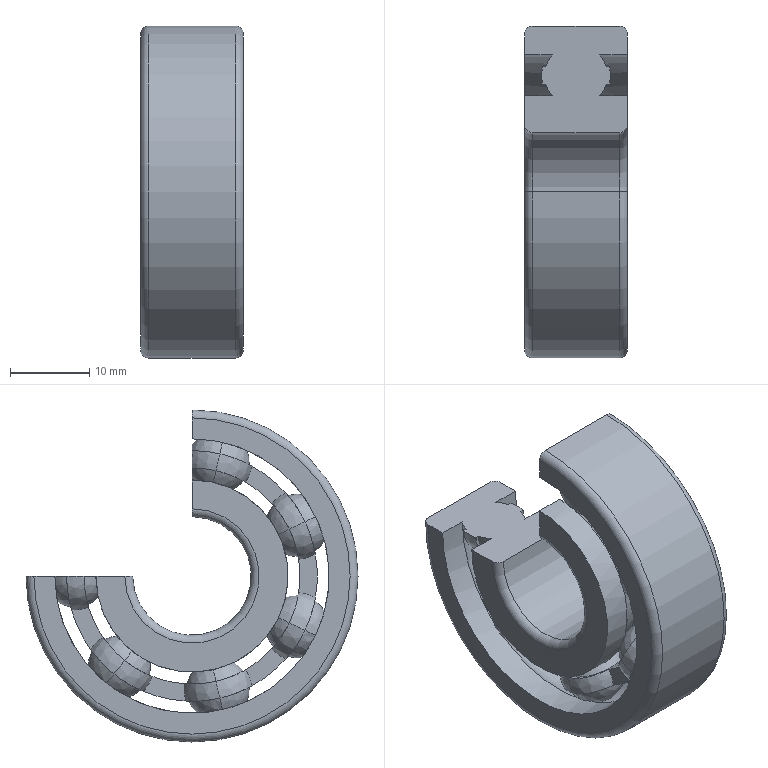Part | STEP file | Bearing 6302 | 1 solid | 92 faces | box 13 x 42 x 42 mm | volume 7890 mm3 | sphere 44 | torus 22 | plane 18 | cylinder 8 | commonest cylinder face diameters 24.3 x2 34.7 x2 15 x1 27.317 x1 31.683 x1 42 x1